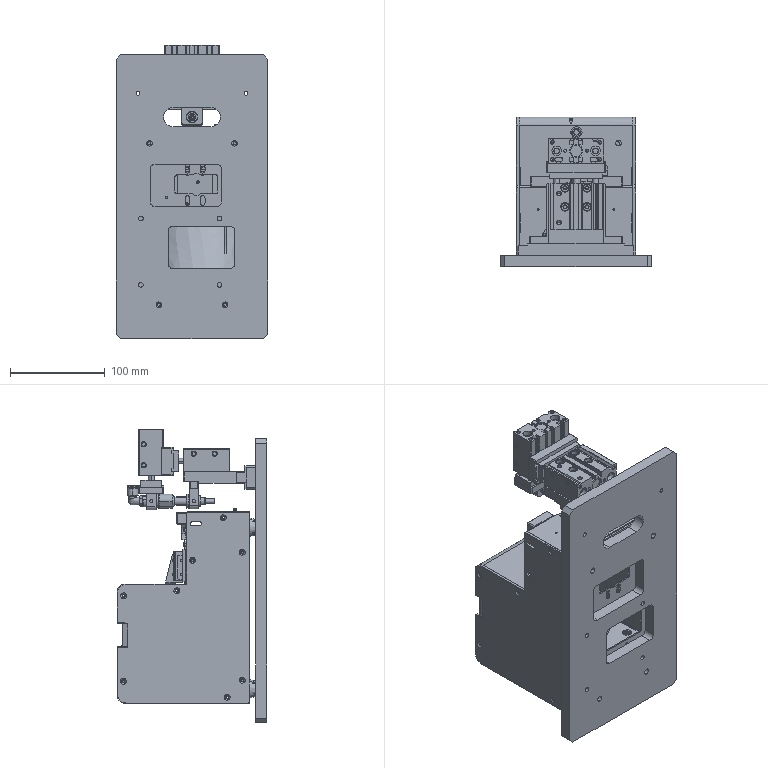Part | SolidWorks | 18 solids | 1952 faces | box 160 x 158.001 x 310 mm | volume 1338981 mm3 | cylinder 828 | plane 794 | cone 280 | spline 31 | torus 19 | commonest cylinder face diameters 3 x77 6 x70 1 x45 4.5 x44 0.8 x40 5 x37